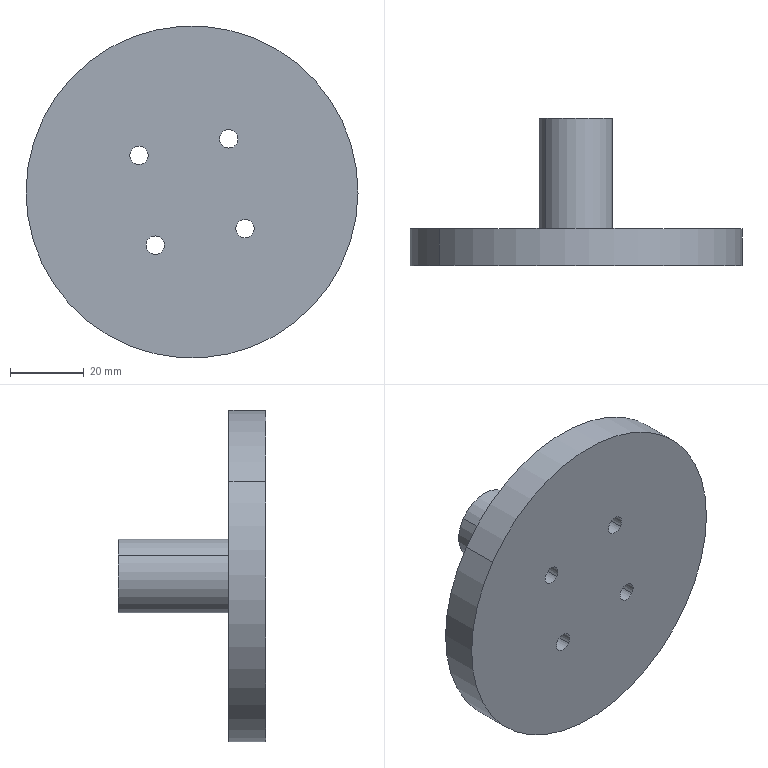Part | STEP file | M6 Tapped Hole的Tapped Hole钻头2 | 1 solid | 15 faces | box 90 x 40 x 90 mm | volume 72257 mm3 | cylinder 12 | plane 3 | commonest cylinder face diameters 5 x8 20 x2 90 x2
STEP:
#1=CARTESIAN_POINT('',(-1570.43,1460.264,2920.934));
#2=VERTEX_POINT('',#1);
#3=CARTESIAN_POINT('',(-1574.543,1460.264,2923.777));
#4=VERTEX_POINT('',#3);
#5=CARTESIAN_POINT('',(-1572.486,1460.264,2922.355));
#6=DIRECTION('',(0.,-1.,0.));
#7=DIRECTION('',(-0.8226,0.,0.5686));
#8=AXIS2_PLACEMENT_3D('',#5,#6,#7);
#9=CIRCLE('',#8,2.5);
#10=EDGE_CURVE('',#2,#4,#9,.T.);
#11=ORIENTED_EDGE('',*,*,#10,.F.);
#12=CARTESIAN_POINT('',(-1570.43,1450.264,2920.934));
#13=VERTEX_POINT('',#12);
#14=CARTESIAN_POINT('',(-1570.43,1450.264,2920.934));
#15=DIRECTION('',(0.,1.,0.));
#16=VECTOR('',#15,1000.);
#17=LINE('',#14,#16);
#18=EDGE_CURVE('',#13,#2,#17,.T.);
#19=ORIENTED_EDGE('',*,*,#18,.F.);
#20=CARTESIAN_POINT('',(-1574.543,1450.264,2923.777));
#21=VERTEX_POINT('',#20);
#22=CARTESIAN_POINT('',(-1572.486,1450.264,2922.355));
#23=DIRECTION('',(0.,-1.,0.));
#24=DIRECTION('',(-0.8226,0.,0.5686));
#25=AXIS2_PLACEMENT_3D('',#22,#23,#24);
#26=CIRCLE('',#25,2.5);
#27=EDGE_CURVE('',#13,#21,#26,.T.);
#28=ORIENTED_EDGE('',*,*,#27,.T.);
#29=CARTESIAN_POINT('',(-1574.543,1450.264,2923.777));
#30=DIRECTION('',(0.,1.,0.));
#31=VECTOR('',#30,1000.);
#32=LINE('',#29,#31);
#33=EDGE_CURVE('',#21,#4,#32,.T.);
#34=ORIENTED_EDGE('',*,*,#33,.T.);
#35=EDGE_LOOP('',(#11,#19,#28,#34));
#36=FACE_OUTER_BOUND('',#35,.T.);
#37=CARTESIAN_POINT('',(-1572.486,1450.264,2922.355));
#38=DIRECTION('',(0.,-1.,0.));
#39=DIRECTION('',(0.8226,0.,-0.5686));
#40=AXIS2_PLACEMENT_3D('',#37,#38,#39);
#41=CYLINDRICAL_SURFACE('',#40,2.5);
#42=ADVANCED_FACE('',(#36),#41,.F.);
#43=CARTESIAN_POINT('',(-1574.875,1460.264,2945.28));
#44=VERTEX_POINT('',#43);
#45=CARTESIAN_POINT('',(-1578.988,1460.264,2948.123));
#46=VERTEX_POINT('',#45);
#47=CARTESIAN_POINT('',(-1576.931,1460.264,2946.701));
#48=DIRECTION('',(0.,-1.,0.));
#49=DIRECTION('',(-0.8226,0.,0.5686));
#50=AXIS2_PLACEMENT_3D('',#47,#48,#49);
#51=CIRCLE('',#50,2.5);
#52=EDGE_CURVE('',#44,#46,#51,.T.);
#53=ORIENTED_EDGE('',*,*,#52,.F.);
#54=CARTESIAN_POINT('',(-1574.875,1450.264,2945.28));
#55=VERTEX_POINT('',#54);
#56=CARTESIAN_POINT('',(-1574.875,1450.264,2945.28));
#57=DIRECTION('',(0.,1.,0.));
#58=VECTOR('',#57,1000.);
#59=LINE('',#56,#58);
#60=EDGE_CURVE('',#55,#44,#59,.T.);
#61=ORIENTED_EDGE('',*,*,#60,.F.);
#62=CARTESIAN_POINT('',(-1578.988,1450.264,2948.123));
#63=VERTEX_POINT('',#62);
#64=CARTESIAN_POINT('',(-1576.931,1450.264,2946.701));
#65=DIRECTION('',(0.,-1.,0.));
#66=DIRECTION('',(-0.8226,0.,0.5686));
#67=AXIS2_PLACEMENT_3D('',#64,#65,#66);
#68=CIRCLE('',#67,2.5);
#69=EDGE_CURVE('',#55,#63,#68,.T.);
#70=ORIENTED_EDGE('',*,*,#69,.T.);
#71=CARTESIAN_POINT('',(-1578.988,1450.264,2948.123));
#72=DIRECTION('',(0.,1.,0.));
#73=VECTOR('',#72,1000.);
#74=LINE('',#71,#73);
#75=EDGE_CURVE('',#63,#46,#74,.T.);
#76=ORIENTED_EDGE('',*,*,#75,.T.);
#77=EDGE_LOOP('',(#53,#61,#70,#76));
#78=FACE_OUTER_BOUND('',#77,.T.);
#79=CARTESIAN_POINT('',(-1576.931,1450.264,2946.701));
#80=DIRECTION('',(0.,-1.,0.));
#81=DIRECTION('',(0.8226,0.,-0.5686));
#82=AXIS2_PLACEMENT_3D('',#79,#80,#81);
#83=CYLINDRICAL_SURFACE('',#82,2.5);
#84=ADVANCED_FACE('',(#78),#83,.F.);
#85=CARTESIAN_POINT('',(-1550.528,1460.264,2949.725));
#86=VERTEX_POINT('',#85);
#87=CARTESIAN_POINT('',(-1554.641,1460.264,2952.568));
#88=VERTEX_POINT('',#87);
#89=CARTESIAN_POINT('',(-1552.585,1460.264,2951.146));
#90=DIRECTION('',(0.,-1.,0.));
#91=DIRECTION('',(-0.8226,0.,0.5686));
#92=AXIS2_PLACEMENT_3D('',#89,#90,#91);
#93=CIRCLE('',#92,2.5);
#94=EDGE_CURVE('',#86,#88,#93,.T.);
#95=ORIENTED_EDGE('',*,*,#94,.F.);
#96=CARTESIAN_POINT('',(-1550.528,1450.264,2949.725));
#97=VERTEX_POINT('',#96);
#98=CARTESIAN_POINT('',(-1550.528,1450.264,2949.725));
#99=DIRECTION('',(0.,1.,0.));
#100=VECTOR('',#99,1000.);
#101=LINE('',#98,#100);
#102=EDGE_CURVE('',#97,#86,#101,.T.);
#103=ORIENTED_EDGE('',*,*,#102,.F.);
#104=CARTESIAN_POINT('',(-1554.641,1450.264,2952.568));
#105=VERTEX_POINT('',#104);
#106=CARTESIAN_POINT('',(-1552.585,1450.264,2951.146));
#107=DIRECTION('',(0.,-1.,0.));
#108=DIRECTION('',(-0.8226,0.,0.5686));
#109=AXIS2_PLACEMENT_3D('',#106,#107,#108);
#110=CIRCLE('',#109,2.5);
#111=EDGE_CURVE('',#97,#105,#110,.T.);
#112=ORIENTED_EDGE('',*,*,#111,.T.);
#113=CARTESIAN_POINT('',(-1554.641,1450.264,2952.568));
#114=DIRECTION('',(0.,1.,0.));
#115=VECTOR('',#114,1000.);
#116=LINE('',#113,#115);
#117=EDGE_CURVE('',#105,#88,#116,.T.);
#118=ORIENTED_EDGE('',*,*,#117,.T.);
#119=EDGE_LOOP('',(#95,#103,#112,#118));
#120=FACE_OUTER_BOUND('',#119,.T.);
#121=CARTESIAN_POINT('',(-1552.585,1450.264,2951.146));
#122=DIRECTION('',(0.,-1.,0.));
#123=DIRECTION('',(0.8226,0.,-0.5686));
#124=AXIS2_PLACEMENT_3D('',#121,#122,#123);
#125=CYLINDRICAL_SURFACE('',#124,2.5);
#126=ADVANCED_FACE('',(#120),#125,.F.);
#127=CARTESIAN_POINT('',(-1546.083,1460.264,2925.378));
#128=VERTEX_POINT('',#127);
#129=CARTESIAN_POINT('',(-1550.196,1460.264,2928.222));
#130=VERTEX_POINT('',#129);
#131=CARTESIAN_POINT('',(-1548.14,1460.264,2926.8));
#132=DIRECTION('',(0.,-1.,0.));
#133=DIRECTION('',(-0.8226,0.,0.5686));
#134=AXIS2_PLACEMENT_3D('',#131,#132,#133);
#135=CIRCLE('',#134,2.5);
#136=EDGE_CURVE('',#128,#130,#135,.T.);
#137=ORIENTED_EDGE('',*,*,#136,.F.);
#138=CARTESIAN_POINT('',(-1546.083,1450.264,2925.378));
#139=VERTEX_POINT('',#138);
#140=CARTESIAN_POINT('',(-1546.083,1450.264,2925.378));
#141=DIRECTION('',(0.,1.,0.));
#142=VECTOR('',#141,1000.);
#143=LINE('',#140,#142);
#144=EDGE_CURVE('',#139,#128,#143,.T.);
#145=ORIENTED_EDGE('',*,*,#144,.F.);
#146=CARTESIAN_POINT('',(-1550.196,1450.264,2928.222));
#147=VERTEX_POINT('',#146);
#148=CARTESIAN_POINT('',(-1548.14,1450.264,2926.8));
#149=DIRECTION('',(0.,-1.,0.));
#150=DIRECTION('',(-0.8226,0.,0.5686));
#151=AXIS2_PLACEMENT_3D('',#148,#149,#150);
#152=CIRCLE('',#151,2.5);
#153=EDGE_CURVE('',#139,#147,#152,.T.);
#154=ORIENTED_EDGE('',*,*,#153,.T.);
#155=CARTESIAN_POINT('',(-1550.196,1450.264,2928.222));
#156=DIRECTION('',(0.,1.,0.));
#157=VECTOR('',#156,1000.);
#158=LINE('',#155,#157);
#159=EDGE_CURVE('',#147,#130,#158,.T.);
#160=ORIENTED_EDGE('',*,*,#159,.T.);
#161=EDGE_LOOP('',(#137,#145,#154,#160));
#162=FACE_OUTER_BOUND('',#161,.T.);
#163=CARTESIAN_POINT('',(-1548.14,1450.264,2926.8));
#164=DIRECTION('',(0.,-1.,0.));
#165=DIRECTION('',(0.8226,0.,-0.5686));
#166=AXIS2_PLACEMENT_3D('',#163,#164,#165);
#167=CYLINDRICAL_SURFACE('',#166,2.5);
#168=ADVANCED_FACE('',(#162),#167,.F.);
#169=CARTESIAN_POINT('',(-1554.309,1490.264,2931.065));
#170=VERTEX_POINT('',#169);
#171=CARTESIAN_POINT('',(-1570.762,1490.264,2942.437));
#172=VERTEX_POINT('',#171);
#173=CARTESIAN_POINT('',(-1562.535,1490.264,2936.751));
#174=DIRECTION('',(0.,1.,0.));
#175=DIRECTION('',(0.8226,0.,-0.5686));
#176=AXIS2_PLACEMENT_3D('',#173,#174,#175);
#177=CIRCLE('',#176,10.);
#178=EDGE_CURVE('',#170,#172,#177,.T.);
#179=ORIENTED_EDGE('',*,*,#178,.F.);
#180=CARTESIAN_POINT('',(-1554.309,1460.264,2931.065));
#181=VERTEX_POINT('',#180);
#182=CARTESIAN_POINT('',(-1554.309,1490.264,2931.065));
#183=DIRECTION('',(0.,1.,0.));
#184=VECTOR('',#183,1000.);
#185=LINE('',#182,#184);
#186=EDGE_CURVE('',#181,#170,#185,.T.);
#187=ORIENTED_EDGE('',*,*,#186,.F.);
#188=CARTESIAN_POINT('',(-1570.762,1460.264,2942.437));
#189=VERTEX_POINT('',#188);
#190=CARTESIAN_POINT('',(-1562.535,1460.264,2936.751));
#191=DIRECTION('',(0.,1.,0.));
#192=DIRECTION('',(0.8226,0.,-0.5686));
#193=AXIS2_PLACEMENT_3D('',#190,#191,#192);
#194=CIRCLE('',#193,10.);
#195=EDGE_CURVE('',#181,#189,#194,.T.);
#196=ORIENTED_EDGE('',*,*,#195,.T.);
#197=CARTESIAN_POINT('',(-1570.762,1490.264,2942.437));
#198=DIRECTION('',(0.,1.,0.));
#199=VECTOR('',#198,1000.);
#200=LINE('',#197,#199);
#201=EDGE_CURVE('',#189,#172,#200,.T.);
#202=ORIENTED_EDGE('',*,*,#201,.T.);
#203=EDGE_LOOP('',(#179,#187,#196,#202));
#204=FACE_OUTER_BOUND('',#203,.T.);
#205=CARTESIAN_POINT('',(-1562.535,1490.264,2936.751));
#206=DIRECTION('',(0.,-1.,0.));
#207=DIRECTION('',(0.8226,0.,-0.5686));
#208=AXIS2_PLACEMENT_3D('',#205,#206,#207);
#209=CYLINDRICAL_SURFACE('',#208,10.);
#210=ADVANCED_FACE('',(#204),#209,.T.);
#211=CARTESIAN_POINT('',(-1525.518,1460.264,2911.163));
#212=VERTEX_POINT('',#211);
#213=CARTESIAN_POINT('',(-1599.553,1460.264,2962.338));
#214=VERTEX_POINT('',#213);
#215=CARTESIAN_POINT('',(-1562.535,1460.264,2936.751));
#216=DIRECTION('',(0.,1.,0.));
#217=DIRECTION('',(0.8226,0.,-0.5686));
#218=AXIS2_PLACEMENT_3D('',#215,#216,#217);
#219=CIRCLE('',#218,45.);
#220=EDGE_CURVE('',#212,#214,#219,.T.);
#221=ORIENTED_EDGE('',*,*,#220,.F.);
#222=CARTESIAN_POINT('',(-1525.518,1450.264,2911.163));
#223=VERTEX_POINT('',#222);
#224=CARTESIAN_POINT('',(-1525.518,1460.264,2911.163));
#225=DIRECTION('',(0.,1.,0.));
#226=VECTOR('',#225,1000.);
#227=LINE('',#224,#226);
#228=EDGE_CURVE('',#223,#212,#227,.T.);
#229=ORIENTED_EDGE('',*,*,#228,.F.);
#230=CARTESIAN_POINT('',(-1599.553,1450.264,2962.338));
#231=VERTEX_POINT('',#230);
#232=CARTESIAN_POINT('',(-1562.535,1450.264,2936.751));
#233=DIRECTION('',(0.,1.,0.));
#234=DIRECTION('',(0.8226,0.,-0.5686));
#235=AXIS2_PLACEMENT_3D('',#232,#233,#234);
#236=CIRCLE('',#235,45.);
#237=EDGE_CURVE('',#223,#231,#236,.T.);
#238=ORIENTED_EDGE('',*,*,#237,.T.);
#239=CARTESIAN_POINT('',(-1599.553,1460.264,2962.338));
#240=DIRECTION('',(0.,1.,0.));
#241=VECTOR('',#240,1000.);
#242=LINE('',#239,#241);
#243=EDGE_CURVE('',#231,#214,#242,.T.);
#244=ORIENTED_EDGE('',*,*,#243,.T.);
#245=EDGE_LOOP('',(#221,#229,#238,#244));
#246=FACE_OUTER_BOUND('',#245,.T.);
#247=CARTESIAN_POINT('',(-1562.535,1460.264,2936.751));
#248=DIRECTION('',(0.,-1.,0.));
#249=DIRECTION('',(0.8226,0.,-0.5686));
#250=AXIS2_PLACEMENT_3D('',#247,#248,#249);
#251=CYLINDRICAL_SURFACE('',#250,45.);
#252=ADVANCED_FACE('',(#246),#251,.T.);
#253=CARTESIAN_POINT('',(-1572.486,1460.264,2922.355));
#254=DIRECTION('',(0.,-1.,0.));
#255=DIRECTION('',(-0.8226,0.,0.5686));
#256=AXIS2_PLACEMENT_3D('',#253,#254,#255);
#257=CIRCLE('',#256,2.5);
#258=EDGE_CURVE('',#4,#2,#257,.T.);
#259=ORIENTED_EDGE('',*,*,#258,.T.);
#260=ORIENTED_EDGE('',*,*,#10,.T.);
#261=EDGE_LOOP('',(#259,#260));
#262=FACE_BOUND('',#261,.T.);
#263=CARTESIAN_POINT('',(-1576.931,1460.264,2946.701));
#264=DIRECTION('',(0.,-1.,0.));
#265=DIRECTION('',(-0.8226,0.,0.5686));
#266=AXIS2_PLACEMENT_3D('',#263,#264,#265);
#267=CIRCLE('',#266,2.5);
#268=EDGE_CURVE('',#46,#44,#267,.T.);
#269=ORIENTED_EDGE('',*,*,#268,.T.);
#270=ORIENTED_EDGE('',*,*,#52,.T.);
#271=EDGE_LOOP('',(#269,#270));
#272=FACE_BOUND('',#271,.T.);
#273=CARTESIAN_POINT('',(-1552.585,1460.264,2951.146));
#274=DIRECTION('',(0.,-1.,0.));
#275=DIRECTION('',(-0.8226,0.,0.5686));
#276=AXIS2_PLACEMENT_3D('',#273,#274,#275);
#277=CIRCLE('',#276,2.5);
#278=EDGE_CURVE('',#88,#86,#277,.T.);
#279=ORIENTED_EDGE('',*,*,#278,.T.);
#280=ORIENTED_EDGE('',*,*,#94,.T.);
#281=EDGE_LOOP('',(#279,#280));
#282=FACE_BOUND('',#281,.T.);
#283=CARTESIAN_POINT('',(-1548.14,1460.264,2926.8));
#284=DIRECTION('',(0.,-1.,0.));
#285=DIRECTION('',(-0.8226,0.,0.5686));
#286=AXIS2_PLACEMENT_3D('',#283,#284,#285);
#287=CIRCLE('',#286,2.5);
#288=EDGE_CURVE('',#130,#128,#287,.T.);
#289=ORIENTED_EDGE('',*,*,#288,.T.);
#290=ORIENTED_EDGE('',*,*,#136,.T.);
#291=EDGE_LOOP('',(#289,#290));
#292=FACE_BOUND('',#291,.T.);
#293=CARTESIAN_POINT('',(-1562.535,1460.264,2936.751));
#294=DIRECTION('',(0.,1.,0.));
#295=DIRECTION('',(0.8226,0.,-0.5686));
#296=AXIS2_PLACEMENT_3D('',#293,#294,#295);
#297=CIRCLE('',#296,45.);
#298=EDGE_CURVE('',#214,#212,#297,.T.);
#299=ORIENTED_EDGE('',*,*,#298,.T.);
#300=ORIENTED_EDGE('',*,*,#220,.T.);
#301=EDGE_LOOP('',(#299,#300));
#302=FACE_OUTER_BOUND('',#301,.T.);
#303=CARTESIAN_POINT('',(-1562.535,1460.264,2936.751));
#304=DIRECTION('',(0.,1.,0.));
#305=DIRECTION('',(0.8226,0.,-0.5686));
#306=AXIS2_PLACEMENT_3D('',#303,#304,#305);
#307=CIRCLE('',#306,10.);
#308=EDGE_CURVE('',#189,#181,#307,.T.);
#309=ORIENTED_EDGE('',*,*,#308,.F.);
#310=ORIENTED_EDGE('',*,*,#195,.F.);
#311=EDGE_LOOP('',(#309,#310));
#312=FACE_BOUND('',#311,.T.);
#313=CARTESIAN_POINT('',(-1562.535,1460.264,2936.751));
#314=DIRECTION('',(0.,1.,0.));
#315=DIRECTION('',(-0.8226,0.,0.5686));
#316=AXIS2_PLACEMENT_3D('',#313,#314,#315);
#317=PLANE('',#316);
#318=ADVANCED_FACE('',(#262,#272,#282,#292,#302,#312),#317,.T.);
#319=ORIENTED_EDGE('',*,*,#228,.T.);
#320=ORIENTED_EDGE('',*,*,#298,.F.);
#321=ORIENTED_EDGE('',*,*,#243,.F.);
#322=CARTESIAN_POINT('',(-1562.535,1450.264,2936.751));
#323=DIRECTION('',(0.,1.,0.));
#324=DIRECTION('',(0.8226,0.,-0.5686));
#325=AXIS2_PLACEMENT_3D('',#322,#323,#324);
#326=CIRCLE('',#325,45.);
#327=EDGE_CURVE('',#231,#223,#326,.T.);
#328=ORIENTED_EDGE('',*,*,#327,.T.);
#329=EDGE_LOOP('',(#319,#320,#321,#328));
#330=FACE_OUTER_BOUND('',#329,.T.);
#331=CARTESIAN_POINT('',(-1562.535,1460.264,2936.751));
#332=DIRECTION('',(0.,-1.,0.));
#333=DIRECTION('',(0.8226,0.,-0.5686));
#334=AXIS2_PLACEMENT_3D('',#331,#332,#333);
#335=CYLINDRICAL_SURFACE('',#334,45.);
#336=ADVANCED_FACE('',(#330),#335,.T.);
#337=CARTESIAN_POINT('',(-1572.486,1450.264,2922.355));
#338=DIRECTION('',(0.,-1.,0.));
#339=DIRECTION('',(-0.8226,0.,0.5686));
#340=AXIS2_PLACEMENT_3D('',#337,#338,#339);
#341=CIRCLE('',#340,2.5);
#342=EDGE_CURVE('',#21,#13,#341,.T.);
#343=ORIENTED_EDGE('',*,*,#342,.F.);
#344=ORIENTED_EDGE('',*,*,#27,.F.);
#345=EDGE_LOOP('',(#343,#344));
#346=FACE_BOUND('',#345,.T.);
#347=CARTESIAN_POINT('',(-1576.931,1450.264,2946.701));
#348=DIRECTION('',(0.,-1.,0.));
#349=DIRECTION('',(-0.8226,0.,0.5686));
#350=AXIS2_PLACEMENT_3D('',#347,#348,#349);
#351=CIRCLE('',#350,2.5);
#352=EDGE_CURVE('',#63,#55,#351,.T.);
#353=ORIENTED_EDGE('',*,*,#352,.F.);
#354=ORIENTED_EDGE('',*,*,#69,.F.);
#355=EDGE_LOOP('',(#353,#354));
#356=FACE_BOUND('',#355,.T.);
#357=CARTESIAN_POINT('',(-1552.585,1450.264,2951.146));
#358=DIRECTION('',(0.,-1.,0.));
#359=DIRECTION('',(-0.8226,0.,0.5686));
#360=AXIS2_PLACEMENT_3D('',#357,#358,#359);
#361=CIRCLE('',#360,2.5);
#362=EDGE_CURVE('',#105,#97,#361,.T.);
#363=ORIENTED_EDGE('',*,*,#362,.F.);
#364=ORIENTED_EDGE('',*,*,#111,.F.);
#365=EDGE_LOOP('',(#363,#364));
#366=FACE_BOUND('',#365,.T.);
#367=CARTESIAN_POINT('',(-1548.14,1450.264,2926.8));
#368=DIRECTION('',(0.,-1.,0.));
#369=DIRECTION('',(-0.8226,0.,0.5686));
#370=AXIS2_PLACEMENT_3D('',#367,#368,#369);
#371=CIRCLE('',#370,2.5);
#372=EDGE_CURVE('',#147,#139,#371,.T.);
#373=ORIENTED_EDGE('',*,*,#372,.F.);
#374=ORIENTED_EDGE('',*,*,#153,.F.);
#375=EDGE_LOOP('',(#373,#374));
#376=FACE_BOUND('',#375,.T.);
#377=ORIENTED_EDGE('',*,*,#327,.F.);
#378=ORIENTED_EDGE('',*,*,#237,.F.);
#379=EDGE_LOOP('',(#377,#378));
#380=FACE_OUTER_BOUND('',#379,.T.);
#381=CARTESIAN_POINT('',(-1562.535,1450.264,2936.751));
#382=DIRECTION('',(0.,1.,0.));
#383=DIRECTION('',(-0.8226,0.,0.5686));
#384=AXIS2_PLACEMENT_3D('',#381,#382,#383);
#385=PLANE('',#384);
#386=ADVANCED_FACE('',(#346,#356,#366,#376,#380),#385,.F.);
#387=ORIENTED_EDGE('',*,*,#186,.T.);
#388=CARTESIAN_POINT('',(-1562.535,1490.264,2936.751));
#389=DIRECTION('',(0.,1.,0.));
#390=DIRECTION('',(0.8226,0.,-0.5686));
#391=AXIS2_PLACEMENT_3D('',#388,#389,#390);
#392=CIRCLE('',#391,10.);
#393=EDGE_CURVE('',#172,#170,#392,.T.);
#394=ORIENTED_EDGE('',*,*,#393,.F.);
#395=ORIENTED_EDGE('',*,*,#201,.F.);
#396=ORIENTED_EDGE('',*,*,#308,.T.);
#397=EDGE_LOOP('',(#387,#394,#395,#396));
#398=FACE_OUTER_BOUND('',#397,.T.);
#399=CARTESIAN_POINT('',(-1562.535,1490.264,2936.751));
#400=DIRECTION('',(0.,-1.,0.));
#401=DIRECTION('',(0.8226,0.,-0.5686));
#402=AXIS2_PLACEMENT_3D('',#399,#400,#401);
#403=CYLINDRICAL_SURFACE('',#402,10.);
#404=ADVANCED_FACE('',(#398),#403,.T.);
#405=ORIENTED_EDGE('',*,*,#393,.T.);
#406=ORIENTED_EDGE('',*,*,#178,.T.);
#407=EDGE_LOOP('',(#405,#406));
#408=FACE_OUTER_BOUND('',#407,.T.);
#409=CARTESIAN_POINT('',(-1562.535,1490.264,2936.751));
#410=DIRECTION('',(0.,1.,0.));
#411=DIRECTION('',(-0.8226,0.,0.5686));
#412=AXIS2_PLACEMENT_3D('',#409,#410,#411);
#413=PLANE('',#412);
#414=ADVANCED_FACE('',(#408),#413,.T.);
#415=ORIENTED_EDGE('',*,*,#144,.T.);
#416=ORIENTED_EDGE('',*,*,#288,.F.);
#417=ORIENTED_EDGE('',*,*,#159,.F.);
#418=ORIENTED_EDGE('',*,*,#372,.T.);
#419=EDGE_LOOP('',(#415,#416,#417,#418));
#420=FACE_OUTER_BOUND('',#419,.T.);
#421=CARTESIAN_POINT('',(-1548.14,1450.264,2926.8));
#422=DIRECTION('',(0.,-1.,0.));
#423=DIRECTION('',(0.8226,0.,-0.5686));
#424=AXIS2_PLACEMENT_3D('',#421,#422,#423);
#425=CYLINDRICAL_SURFACE('',#424,2.5);
#426=ADVANCED_FACE('',(#420),#425,.F.);
#427=ORIENTED_EDGE('',*,*,#102,.T.);
#428=ORIENTED_EDGE('',*,*,#278,.F.);
#429=ORIENTED_EDGE('',*,*,#117,.F.);
#430=ORIENTED_EDGE('',*,*,#362,.T.);
#431=EDGE_LOOP('',(#427,#428,#429,#430));
#432=FACE_OUTER_BOUND('',#431,.T.);
#433=CARTESIAN_POINT('',(-1552.585,1450.264,2951.146));
#434=DIRECTION('',(0.,-1.,0.));
#435=DIRECTION('',(0.8226,0.,-0.5686));
#436=AXIS2_PLACEMENT_3D('',#433,#434,#435);
#437=CYLINDRICAL_SURFACE('',#436,2.5);
#438=ADVANCED_FACE('',(#432),#437,.F.);
#439=ORIENTED_EDGE('',*,*,#60,.T.);
#440=ORIENTED_EDGE('',*,*,#268,.F.);
#441=ORIENTED_EDGE('',*,*,#75,.F.);
#442=ORIENTED_EDGE('',*,*,#352,.T.);
#443=EDGE_LOOP('',(#439,#440,#441,#442));
#444=FACE_OUTER_BOUND('',#443,.T.);
#445=CARTESIAN_POINT('',(-1576.931,1450.264,2946.701));
#446=DIRECTION('',(0.,-1.,0.));
#447=DIRECTION('',(0.8226,0.,-0.5686));
#448=AXIS2_PLACEMENT_3D('',#445,#446,#447);
#449=CYLINDRICAL_SURFACE('',#448,2.5);
#450=ADVANCED_FACE('',(#444),#449,.F.);
#451=ORIENTED_EDGE('',*,*,#18,.T.);
#452=ORIENTED_EDGE('',*,*,#258,.F.);
#453=ORIENTED_EDGE('',*,*,#33,.F.);
#454=ORIENTED_EDGE('',*,*,#342,.T.);
#455=EDGE_LOOP('',(#451,#452,#453,#454));
#456=FACE_OUTER_BOUND('',#455,.T.);
#457=CARTESIAN_POINT('',(-1572.486,1450.264,2922.355));
#458=DIRECTION('',(0.,-1.,0.));
#459=DIRECTION('',(0.8226,0.,-0.5686));
#460=AXIS2_PLACEMENT_3D('',#457,#458,#459);
#461=CYLINDRICAL_SURFACE('',#460,2.5);
#462=ADVANCED_FACE('',(#456),#461,.F.);
#463=CLOSED_SHELL('',(#42,#84,#126,#168,#210,#252,#318,#336,#386,#404,#414,#426,#438,#450,#462));
#464=MANIFOLD_SOLID_BREP('',#463);
#465=CARTESIAN_POINT('',(0.,0.,0.));
#466=DIRECTION('',(0.,0.,1.));
#467=DIRECTION('',(1.,0.,0.));
#468=AXIS2_PLACEMENT_3D('',#465,#466,#467);
#469=(LENGTH_UNIT()NAMED_UNIT(*)SI_UNIT(.MILLI.,.METRE.));
#470=UNCERTAINTY_MEASURE_WITH_UNIT(LENGTH_MEASURE(0.00001),#469,'','');
#471=(NAMED_UNIT(*)PLANE_ANGLE_UNIT()SI_UNIT($,.RADIAN.));
#472=(NAMED_UNIT(*)SI_UNIT($,.STERADIAN.)SOLID_ANGLE_UNIT());
#473=(GEOMETRIC_REPRESENTATION_CONTEXT(3)GLOBAL_UNCERTAINTY_ASSIGNED_CONTEXT((#470))GLOBAL_UNIT_ASSIGNED_CONTEXT((#469,#471,#472))REPRESENTATION_CONTEXT('',''));
#474=ADVANCED_BREP_SHAPE_REPRESENTATION('',(#464,#468),#473);